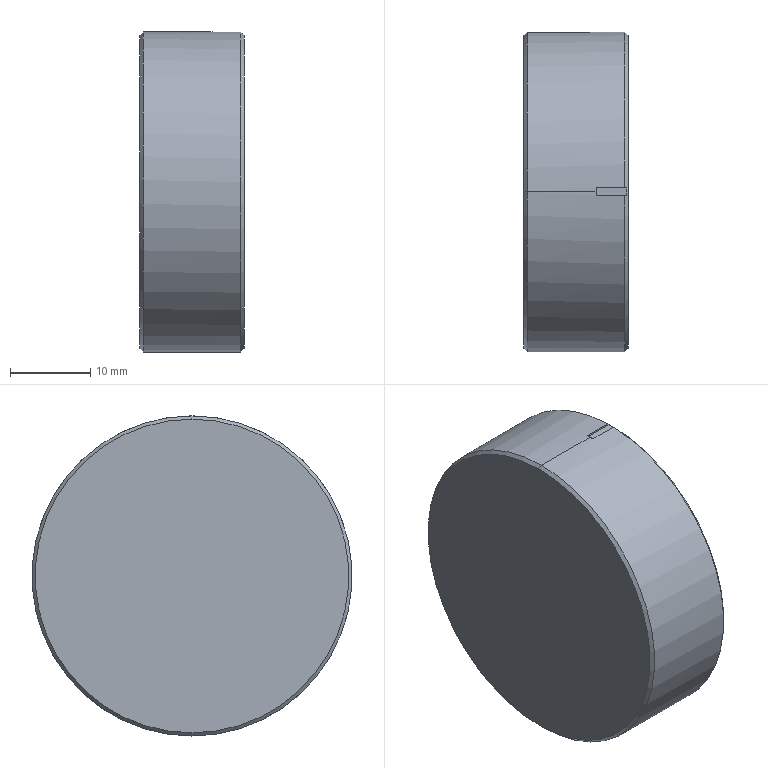Part | STEP file | ASND-0110-IRB120_Link6_rev0 | 1 solid | 37 faces | box 13 x 40 x 40 mm | volume 13678 mm3 | cone 16 | cylinder 14 | plane 7 | commonest cylinder face diameters 4.2 x8 5 x2 20 x2 40 x2